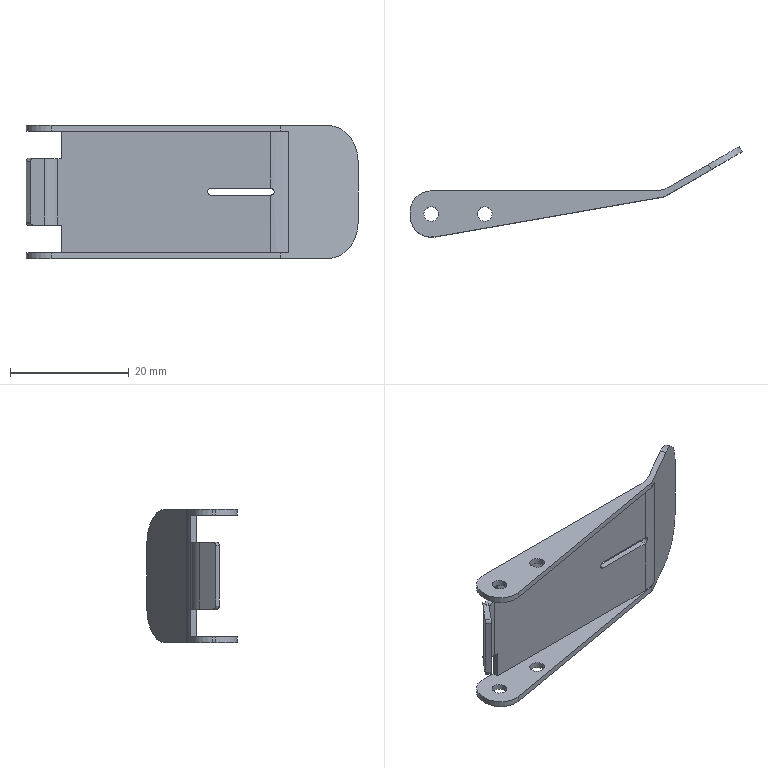Part | SolidWorks | features BaseBody 1 | 1 solid | 52 faces | box 56.004 x 15.265 x 22.5 mm | volume 1517 mm3 | plane 29 | cylinder 23 | commonest cylinder face diameters 2.5 x8 7.2 x4 1.2 x3 12 x3 1 x2 6 x1